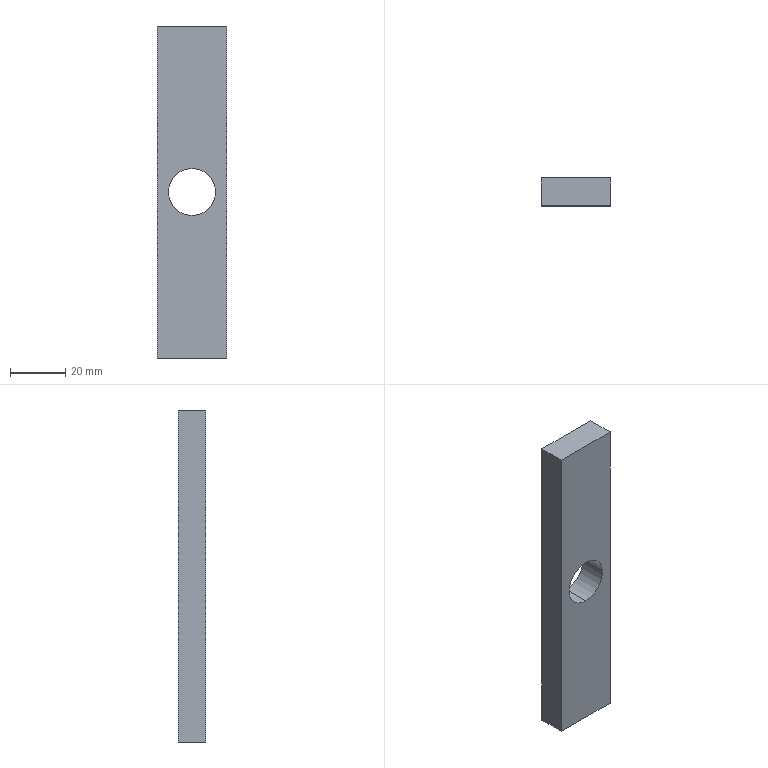Part | SolidWorks | features ICE 2, Extrusion 1 | 1 solid | 14 faces | box 25 x 10 x 120 mm | volume 26926 mm3 | plane 8 | cylinder 6 | commonest cylinder face diameters 16 x4 17 x2
STEP:
#1=CARTESIAN_POINT('',(0.,0.,-8.5));
#2=VERTEX_POINT('',#1);
#3=CARTESIAN_POINT('',(0.,0.,8.5));
#4=VERTEX_POINT('',#3);
#5=CARTESIAN_POINT('',(0.,0.,0.));
#6=DIRECTION('',(0.,1.,0.));
#7=DIRECTION('',(0.,0.,-1.));
#8=AXIS2_PLACEMENT_3D('',#5,#6,#7);
#9=CIRCLE('',#8,8.5);
#10=EDGE_CURVE('',#2,#4,#9,.T.);
#11=ORIENTED_EDGE('',*,*,#10,.F.);
#12=CARTESIAN_POINT('',(0.,10.,-8.5));
#13=VERTEX_POINT('',#12);
#14=CARTESIAN_POINT('',(0.,-0.001,-8.5));
#15=DIRECTION('',(0.,1.,0.));
#16=VECTOR('',#15,1000.);
#17=LINE('',#14,#16);
#18=EDGE_CURVE('',#2,#13,#17,.T.);
#19=ORIENTED_EDGE('',*,*,#18,.T.);
#20=CARTESIAN_POINT('',(0.,10.,8.5));
#21=VERTEX_POINT('',#20);
#22=CARTESIAN_POINT('',(0.,10.,0.));
#23=DIRECTION('',(0.,1.,0.));
#24=DIRECTION('',(0.,0.,1.));
#25=AXIS2_PLACEMENT_3D('',#22,#23,#24);
#26=CIRCLE('',#25,8.5);
#27=EDGE_CURVE('',#13,#21,#26,.T.);
#28=ORIENTED_EDGE('',*,*,#27,.T.);
#29=CARTESIAN_POINT('',(0.,-0.001,8.5));
#30=DIRECTION('',(0.,1.,0.));
#31=VECTOR('',#30,1000.);
#32=LINE('',#29,#31);
#33=EDGE_CURVE('',#4,#21,#32,.T.);
#34=ORIENTED_EDGE('',*,*,#33,.F.);
#35=EDGE_LOOP('',(#11,#19,#28,#34));
#36=FACE_OUTER_BOUND('',#35,.T.);
#37=CARTESIAN_POINT('',(0.,-0.001,0.));
#38=DIRECTION('',(0.,1.,0.));
#39=DIRECTION('',(0.,0.,1.));
#40=AXIS2_PLACEMENT_3D('',#37,#38,#39);
#41=CYLINDRICAL_SURFACE('',#40,8.5);
#42=ADVANCED_FACE('',(#36),#41,.F.);
#43=CARTESIAN_POINT('',(0.,8.,-54.));
#44=VERTEX_POINT('',#43);
#45=CARTESIAN_POINT('',(0.,8.,-38.));
#46=VERTEX_POINT('',#45);
#47=CARTESIAN_POINT('',(0.,8.,-46.));
#48=DIRECTION('',(0.,1.,0.));
#49=DIRECTION('',(0.,0.,1.));
#50=AXIS2_PLACEMENT_3D('',#47,#48,#49);
#51=CIRCLE('',#50,8.);
#52=EDGE_CURVE('',#44,#46,#51,.T.);
#53=ORIENTED_EDGE('',*,*,#52,.F.);
#54=CARTESIAN_POINT('',(0.,10.,-54.));
#55=VERTEX_POINT('',#54);
#56=CARTESIAN_POINT('',(0.,8.,-54.));
#57=DIRECTION('',(0.,1.,0.));
#58=VECTOR('',#57,1000.);
#59=LINE('',#56,#58);
#60=EDGE_CURVE('',#44,#55,#59,.T.);
#61=ORIENTED_EDGE('',*,*,#60,.T.);
#62=CARTESIAN_POINT('',(0.,10.,-38.));
#63=VERTEX_POINT('',#62);
#64=CARTESIAN_POINT('',(0.,10.,-46.));
#65=DIRECTION('',(0.,1.,0.));
#66=DIRECTION('',(0.,0.,1.));
#67=AXIS2_PLACEMENT_3D('',#64,#65,#66);
#68=CIRCLE('',#67,8.);
#69=EDGE_CURVE('',#55,#63,#68,.T.);
#70=ORIENTED_EDGE('',*,*,#69,.T.);
#71=CARTESIAN_POINT('',(0.,8.,-38.));
#72=DIRECTION('',(0.,1.,0.));
#73=VECTOR('',#72,1000.);
#74=LINE('',#71,#73);
#75=EDGE_CURVE('',#46,#63,#74,.T.);
#76=ORIENTED_EDGE('',*,*,#75,.F.);
#77=EDGE_LOOP('',(#53,#61,#70,#76));
#78=FACE_OUTER_BOUND('',#77,.T.);
#79=CARTESIAN_POINT('',(0.,8.,-46.));
#80=DIRECTION('',(0.,1.,0.));
#81=DIRECTION('',(0.,0.,1.));
#82=AXIS2_PLACEMENT_3D('',#79,#80,#81);
#83=CYLINDRICAL_SURFACE('',#82,8.);
#84=ADVANCED_FACE('',(#78),#83,.F.);
#85=CARTESIAN_POINT('',(0.,8.,38.));
#86=VERTEX_POINT('',#85);
#87=CARTESIAN_POINT('',(0.,8.,54.));
#88=VERTEX_POINT('',#87);
#89=CARTESIAN_POINT('',(0.,8.,46.));
#90=DIRECTION('',(0.,1.,0.));
#91=DIRECTION('',(0.,0.,1.));
#92=AXIS2_PLACEMENT_3D('',#89,#90,#91);
#93=CIRCLE('',#92,8.);
#94=EDGE_CURVE('',#86,#88,#93,.T.);
#95=ORIENTED_EDGE('',*,*,#94,.F.);
#96=CARTESIAN_POINT('',(0.,10.,38.));
#97=VERTEX_POINT('',#96);
#98=CARTESIAN_POINT('',(0.,8.,38.));
#99=DIRECTION('',(0.,1.,0.));
#100=VECTOR('',#99,1000.);
#101=LINE('',#98,#100);
#102=EDGE_CURVE('',#86,#97,#101,.T.);
#103=ORIENTED_EDGE('',*,*,#102,.T.);
#104=CARTESIAN_POINT('',(0.,10.,54.));
#105=VERTEX_POINT('',#104);
#106=CARTESIAN_POINT('',(0.,10.,46.));
#107=DIRECTION('',(0.,1.,0.));
#108=DIRECTION('',(0.,0.,1.));
#109=AXIS2_PLACEMENT_3D('',#106,#107,#108);
#110=CIRCLE('',#109,8.);
#111=EDGE_CURVE('',#97,#105,#110,.T.);
#112=ORIENTED_EDGE('',*,*,#111,.T.);
#113=CARTESIAN_POINT('',(0.,8.,54.));
#114=DIRECTION('',(0.,1.,0.));
#115=VECTOR('',#114,1000.);
#116=LINE('',#113,#115);
#117=EDGE_CURVE('',#88,#105,#116,.T.);
#118=ORIENTED_EDGE('',*,*,#117,.F.);
#119=EDGE_LOOP('',(#95,#103,#112,#118));
#120=FACE_OUTER_BOUND('',#119,.T.);
#121=CARTESIAN_POINT('',(0.,8.,46.));
#122=DIRECTION('',(0.,1.,0.));
#123=DIRECTION('',(0.,0.,1.));
#124=AXIS2_PLACEMENT_3D('',#121,#122,#123);
#125=CYLINDRICAL_SURFACE('',#124,8.);
#126=ADVANCED_FACE('',(#120),#125,.F.);
#127=CARTESIAN_POINT('',(12.5,0.,60.));
#128=VERTEX_POINT('',#127);
#129=CARTESIAN_POINT('',(12.5,0.,-60.));
#130=VERTEX_POINT('',#129);
#131=CARTESIAN_POINT('',(12.5,0.,60.));
#132=DIRECTION('',(0.,0.,-1.));
#133=VECTOR('',#132,1000.);
#134=LINE('',#131,#133);
#135=EDGE_CURVE('',#128,#130,#134,.T.);
#136=ORIENTED_EDGE('',*,*,#135,.T.);
#137=CARTESIAN_POINT('',(12.5,10.,-60.));
#138=VERTEX_POINT('',#137);
#139=CARTESIAN_POINT('',(12.5,10.,-60.));
#140=DIRECTION('',(0.,-1.,0.));
#141=VECTOR('',#140,1000.);
#142=LINE('',#139,#141);
#143=EDGE_CURVE('',#138,#130,#142,.T.);
#144=ORIENTED_EDGE('',*,*,#143,.F.);
#145=CARTESIAN_POINT('',(12.5,10.,60.));
#146=VERTEX_POINT('',#145);
#147=CARTESIAN_POINT('',(12.5,10.,60.));
#148=DIRECTION('',(0.,0.,-1.));
#149=VECTOR('',#148,1000.);
#150=LINE('',#147,#149);
#151=EDGE_CURVE('',#146,#138,#150,.T.);
#152=ORIENTED_EDGE('',*,*,#151,.F.);
#153=CARTESIAN_POINT('',(12.5,10.,60.));
#154=DIRECTION('',(0.,-1.,0.));
#155=VECTOR('',#154,1000.);
#156=LINE('',#153,#155);
#157=EDGE_CURVE('',#146,#128,#156,.T.);
#158=ORIENTED_EDGE('',*,*,#157,.T.);
#159=EDGE_LOOP('',(#136,#144,#152,#158));
#160=FACE_OUTER_BOUND('',#159,.T.);
#161=CARTESIAN_POINT('',(12.5,10.,60.));
#162=DIRECTION('',(-1.,0.,0.));
#163=DIRECTION('',(0.,0.,1.));
#164=AXIS2_PLACEMENT_3D('',#161,#162,#163);
#165=PLANE('',#164);
#166=ADVANCED_FACE('',(#160),#165,.F.);
#167=CARTESIAN_POINT('',(-12.5,0.,-60.));
#168=VERTEX_POINT('',#167);
#169=CARTESIAN_POINT('',(-12.5,0.,-60.));
#170=DIRECTION('',(-1.,0.,0.));
#171=VECTOR('',#170,1000.);
#172=LINE('',#169,#171);
#173=EDGE_CURVE('',#130,#168,#172,.T.);
#174=ORIENTED_EDGE('',*,*,#173,.T.);
#175=CARTESIAN_POINT('',(-12.5,10.,-60.));
#176=VERTEX_POINT('',#175);
#177=CARTESIAN_POINT('',(-12.5,10.,-60.));
#178=DIRECTION('',(0.,-1.,0.));
#179=VECTOR('',#178,1000.);
#180=LINE('',#177,#179);
#181=EDGE_CURVE('',#176,#168,#180,.T.);
#182=ORIENTED_EDGE('',*,*,#181,.F.);
#183=CARTESIAN_POINT('',(-12.5,10.,-60.));
#184=DIRECTION('',(-1.,0.,0.));
#185=VECTOR('',#184,1000.);
#186=LINE('',#183,#185);
#187=EDGE_CURVE('',#138,#176,#186,.T.);
#188=ORIENTED_EDGE('',*,*,#187,.F.);
#189=ORIENTED_EDGE('',*,*,#143,.T.);
#190=EDGE_LOOP('',(#174,#182,#188,#189));
#191=FACE_OUTER_BOUND('',#190,.T.);
#192=CARTESIAN_POINT('',(-12.5,10.,-60.));
#193=DIRECTION('',(0.,0.,1.));
#194=DIRECTION('',(1.,0.,0.));
#195=AXIS2_PLACEMENT_3D('',#192,#193,#194);
#196=PLANE('',#195);
#197=ADVANCED_FACE('',(#191),#196,.F.);
#198=CARTESIAN_POINT('',(-12.5,0.,60.));
#199=VERTEX_POINT('',#198);
#200=CARTESIAN_POINT('',(-12.5,0.,60.));
#201=DIRECTION('',(0.,0.,1.));
#202=VECTOR('',#201,1000.);
#203=LINE('',#200,#202);
#204=EDGE_CURVE('',#168,#199,#203,.T.);
#205=ORIENTED_EDGE('',*,*,#204,.T.);
#206=CARTESIAN_POINT('',(-12.5,10.,60.));
#207=VERTEX_POINT('',#206);
#208=CARTESIAN_POINT('',(-12.5,10.,60.));
#209=DIRECTION('',(0.,-1.,0.));
#210=VECTOR('',#209,1000.);
#211=LINE('',#208,#210);
#212=EDGE_CURVE('',#207,#199,#211,.T.);
#213=ORIENTED_EDGE('',*,*,#212,.F.);
#214=CARTESIAN_POINT('',(-12.5,10.,60.));
#215=DIRECTION('',(0.,0.,1.));
#216=VECTOR('',#215,1000.);
#217=LINE('',#214,#216);
#218=EDGE_CURVE('',#176,#207,#217,.T.);
#219=ORIENTED_EDGE('',*,*,#218,.F.);
#220=ORIENTED_EDGE('',*,*,#181,.T.);
#221=EDGE_LOOP('',(#205,#213,#219,#220));
#222=FACE_OUTER_BOUND('',#221,.T.);
#223=CARTESIAN_POINT('',(-12.5,10.,60.));
#224=DIRECTION('',(1.,0.,0.));
#225=DIRECTION('',(0.,0.,-1.));
#226=AXIS2_PLACEMENT_3D('',#223,#224,#225);
#227=PLANE('',#226);
#228=ADVANCED_FACE('',(#222),#227,.F.);
#229=CARTESIAN_POINT('',(-12.5,0.,60.));
#230=DIRECTION('',(1.,0.,0.));
#231=VECTOR('',#230,1000.);
#232=LINE('',#229,#231);
#233=EDGE_CURVE('',#199,#128,#232,.T.);
#234=ORIENTED_EDGE('',*,*,#233,.T.);
#235=ORIENTED_EDGE('',*,*,#157,.F.);
#236=CARTESIAN_POINT('',(-12.5,10.,60.));
#237=DIRECTION('',(1.,0.,0.));
#238=VECTOR('',#237,1000.);
#239=LINE('',#236,#238);
#240=EDGE_CURVE('',#207,#146,#239,.T.);
#241=ORIENTED_EDGE('',*,*,#240,.F.);
#242=ORIENTED_EDGE('',*,*,#212,.T.);
#243=EDGE_LOOP('',(#234,#235,#241,#242));
#244=FACE_OUTER_BOUND('',#243,.T.);
#245=CARTESIAN_POINT('',(-12.5,10.,60.));
#246=DIRECTION('',(0.,0.,-1.));
#247=DIRECTION('',(-1.,0.,0.));
#248=AXIS2_PLACEMENT_3D('',#245,#246,#247);
#249=PLANE('',#248);
#250=ADVANCED_FACE('',(#244),#249,.F.);
#251=CARTESIAN_POINT('',(0.,10.,0.));
#252=DIRECTION('',(0.,1.,0.));
#253=DIRECTION('',(0.,0.,1.));
#254=AXIS2_PLACEMENT_3D('',#251,#252,#253);
#255=CIRCLE('',#254,8.5);
#256=EDGE_CURVE('',#21,#13,#255,.T.);
#257=ORIENTED_EDGE('',*,*,#256,.F.);
#258=ORIENTED_EDGE('',*,*,#27,.F.);
#259=EDGE_LOOP('',(#257,#258));
#260=FACE_BOUND('',#259,.T.);
#261=CARTESIAN_POINT('',(0.,10.,-46.));
#262=DIRECTION('',(0.,1.,0.));
#263=DIRECTION('',(0.,0.,1.));
#264=AXIS2_PLACEMENT_3D('',#261,#262,#263);
#265=CIRCLE('',#264,8.);
#266=EDGE_CURVE('',#63,#55,#265,.T.);
#267=ORIENTED_EDGE('',*,*,#266,.F.);
#268=ORIENTED_EDGE('',*,*,#69,.F.);
#269=EDGE_LOOP('',(#267,#268));
#270=FACE_BOUND('',#269,.T.);
#271=CARTESIAN_POINT('',(0.,10.,46.));
#272=DIRECTION('',(0.,1.,0.));
#273=DIRECTION('',(0.,0.,1.));
#274=AXIS2_PLACEMENT_3D('',#271,#272,#273);
#275=CIRCLE('',#274,8.);
#276=EDGE_CURVE('',#105,#97,#275,.T.);
#277=ORIENTED_EDGE('',*,*,#276,.F.);
#278=ORIENTED_EDGE('',*,*,#111,.F.);
#279=EDGE_LOOP('',(#277,#278));
#280=FACE_BOUND('',#279,.T.);
#281=ORIENTED_EDGE('',*,*,#151,.T.);
#282=ORIENTED_EDGE('',*,*,#187,.T.);
#283=ORIENTED_EDGE('',*,*,#218,.T.);
#284=ORIENTED_EDGE('',*,*,#240,.T.);
#285=EDGE_LOOP('',(#281,#282,#283,#284));
#286=FACE_OUTER_BOUND('',#285,.T.);
#287=CARTESIAN_POINT('',(0.,10.,0.));
#288=DIRECTION('',(0.,-1.,0.));
#289=DIRECTION('',(0.,0.,-1.));
#290=AXIS2_PLACEMENT_3D('',#287,#288,#289);
#291=PLANE('',#290);
#292=ADVANCED_FACE('',(#260,#270,#280,#286),#291,.F.);
#293=CARTESIAN_POINT('',(0.,0.,0.));
#294=DIRECTION('',(0.,1.,0.));
#295=DIRECTION('',(0.,0.,-1.));
#296=AXIS2_PLACEMENT_3D('',#293,#294,#295);
#297=CIRCLE('',#296,8.5);
#298=EDGE_CURVE('',#4,#2,#297,.T.);
#299=ORIENTED_EDGE('',*,*,#298,.T.);
#300=ORIENTED_EDGE('',*,*,#10,.T.);
#301=EDGE_LOOP('',(#299,#300));
#302=FACE_BOUND('',#301,.T.);
#303=ORIENTED_EDGE('',*,*,#135,.F.);
#304=ORIENTED_EDGE('',*,*,#233,.F.);
#305=ORIENTED_EDGE('',*,*,#204,.F.);
#306=ORIENTED_EDGE('',*,*,#173,.F.);
#307=EDGE_LOOP('',(#303,#304,#305,#306));
#308=FACE_OUTER_BOUND('',#307,.T.);
#309=CARTESIAN_POINT('',(0.,0.,0.));
#310=DIRECTION('',(0.,-1.,0.));
#311=DIRECTION('',(0.,0.,-1.));
#312=AXIS2_PLACEMENT_3D('',#309,#310,#311);
#313=PLANE('',#312);
#314=ADVANCED_FACE('',(#302,#308),#313,.T.);
#315=ORIENTED_EDGE('',*,*,#102,.F.);
#316=CARTESIAN_POINT('',(0.,8.,46.));
#317=DIRECTION('',(0.,1.,0.));
#318=DIRECTION('',(0.,0.,1.));
#319=AXIS2_PLACEMENT_3D('',#316,#317,#318);
#320=CIRCLE('',#319,8.);
#321=EDGE_CURVE('',#88,#86,#320,.T.);
#322=ORIENTED_EDGE('',*,*,#321,.F.);
#323=ORIENTED_EDGE('',*,*,#117,.T.);
#324=ORIENTED_EDGE('',*,*,#276,.T.);
#325=EDGE_LOOP('',(#315,#322,#323,#324));
#326=FACE_OUTER_BOUND('',#325,.T.);
#327=CARTESIAN_POINT('',(0.,8.,46.));
#328=DIRECTION('',(0.,1.,0.));
#329=DIRECTION('',(0.,0.,1.));
#330=AXIS2_PLACEMENT_3D('',#327,#328,#329);
#331=CYLINDRICAL_SURFACE('',#330,8.);
#332=ADVANCED_FACE('',(#326),#331,.F.);
#333=ORIENTED_EDGE('',*,*,#321,.T.);
#334=ORIENTED_EDGE('',*,*,#94,.T.);
#335=EDGE_LOOP('',(#333,#334));
#336=FACE_OUTER_BOUND('',#335,.T.);
#337=CARTESIAN_POINT('',(0.,8.,46.));
#338=DIRECTION('',(0.,1.,0.));
#339=DIRECTION('',(0.,0.,1.));
#340=AXIS2_PLACEMENT_3D('',#337,#338,#339);
#341=PLANE('',#340);
#342=ADVANCED_FACE('',(#336),#341,.T.);
#343=ORIENTED_EDGE('',*,*,#60,.F.);
#344=CARTESIAN_POINT('',(0.,8.,-46.));
#345=DIRECTION('',(0.,1.,0.));
#346=DIRECTION('',(0.,0.,1.));
#347=AXIS2_PLACEMENT_3D('',#344,#345,#346);
#348=CIRCLE('',#347,8.);
#349=EDGE_CURVE('',#46,#44,#348,.T.);
#350=ORIENTED_EDGE('',*,*,#349,.F.);
#351=ORIENTED_EDGE('',*,*,#75,.T.);
#352=ORIENTED_EDGE('',*,*,#266,.T.);
#353=EDGE_LOOP('',(#343,#350,#351,#352));
#354=FACE_OUTER_BOUND('',#353,.T.);
#355=CARTESIAN_POINT('',(0.,8.,-46.));
#356=DIRECTION('',(0.,1.,0.));
#357=DIRECTION('',(0.,0.,1.));
#358=AXIS2_PLACEMENT_3D('',#355,#356,#357);
#359=CYLINDRICAL_SURFACE('',#358,8.);
#360=ADVANCED_FACE('',(#354),#359,.F.);
#361=ORIENTED_EDGE('',*,*,#349,.T.);
#362=ORIENTED_EDGE('',*,*,#52,.T.);
#363=EDGE_LOOP('',(#361,#362));
#364=FACE_OUTER_BOUND('',#363,.T.);
#365=CARTESIAN_POINT('',(0.,8.,-46.));
#366=DIRECTION('',(0.,1.,0.));
#367=DIRECTION('',(0.,0.,1.));
#368=AXIS2_PLACEMENT_3D('',#365,#366,#367);
#369=PLANE('',#368);
#370=ADVANCED_FACE('',(#364),#369,.T.);
#371=ORIENTED_EDGE('',*,*,#18,.F.);
#372=ORIENTED_EDGE('',*,*,#298,.F.);
#373=ORIENTED_EDGE('',*,*,#33,.T.);
#374=ORIENTED_EDGE('',*,*,#256,.T.);
#375=EDGE_LOOP('',(#371,#372,#373,#374));
#376=FACE_OUTER_BOUND('',#375,.T.);
#377=CARTESIAN_POINT('',(0.,-0.001,0.));
#378=DIRECTION('',(0.,1.,0.));
#379=DIRECTION('',(0.,0.,1.));
#380=AXIS2_PLACEMENT_3D('',#377,#378,#379);
#381=CYLINDRICAL_SURFACE('',#380,8.5);
#382=ADVANCED_FACE('',(#376),#381,.F.);
#383=CLOSED_SHELL('',(#42,#84,#126,#166,#197,#228,#250,#292,#314,#332,#342,#360,#370,#382));
#384=MANIFOLD_SOLID_BREP('',#383);
#385=CARTESIAN_POINT('',(0.,0.,0.));
#386=DIRECTION('',(0.,0.,1.));
#387=DIRECTION('',(1.,0.,0.));
#388=AXIS2_PLACEMENT_3D('',#385,#386,#387);
#389=(LENGTH_UNIT()NAMED_UNIT(*)SI_UNIT(.MILLI.,.METRE.));
#390=UNCERTAINTY_MEASURE_WITH_UNIT(LENGTH_MEASURE(0.00001),#389,'','');
#391=(NAMED_UNIT(*)PLANE_ANGLE_UNIT()SI_UNIT($,.RADIAN.));
#392=(NAMED_UNIT(*)SI_UNIT($,.STERADIAN.)SOLID_ANGLE_UNIT());
#393=(GEOMETRIC_REPRESENTATION_CONTEXT(3)GLOBAL_UNCERTAINTY_ASSIGNED_CONTEXT((#390))GLOBAL_UNIT_ASSIGNED_CONTEXT((#389,#391,#392))REPRESENTATION_CONTEXT('',''));
#394=ADVANCED_BREP_SHAPE_REPRESENTATION('',(#384,#388),#393);